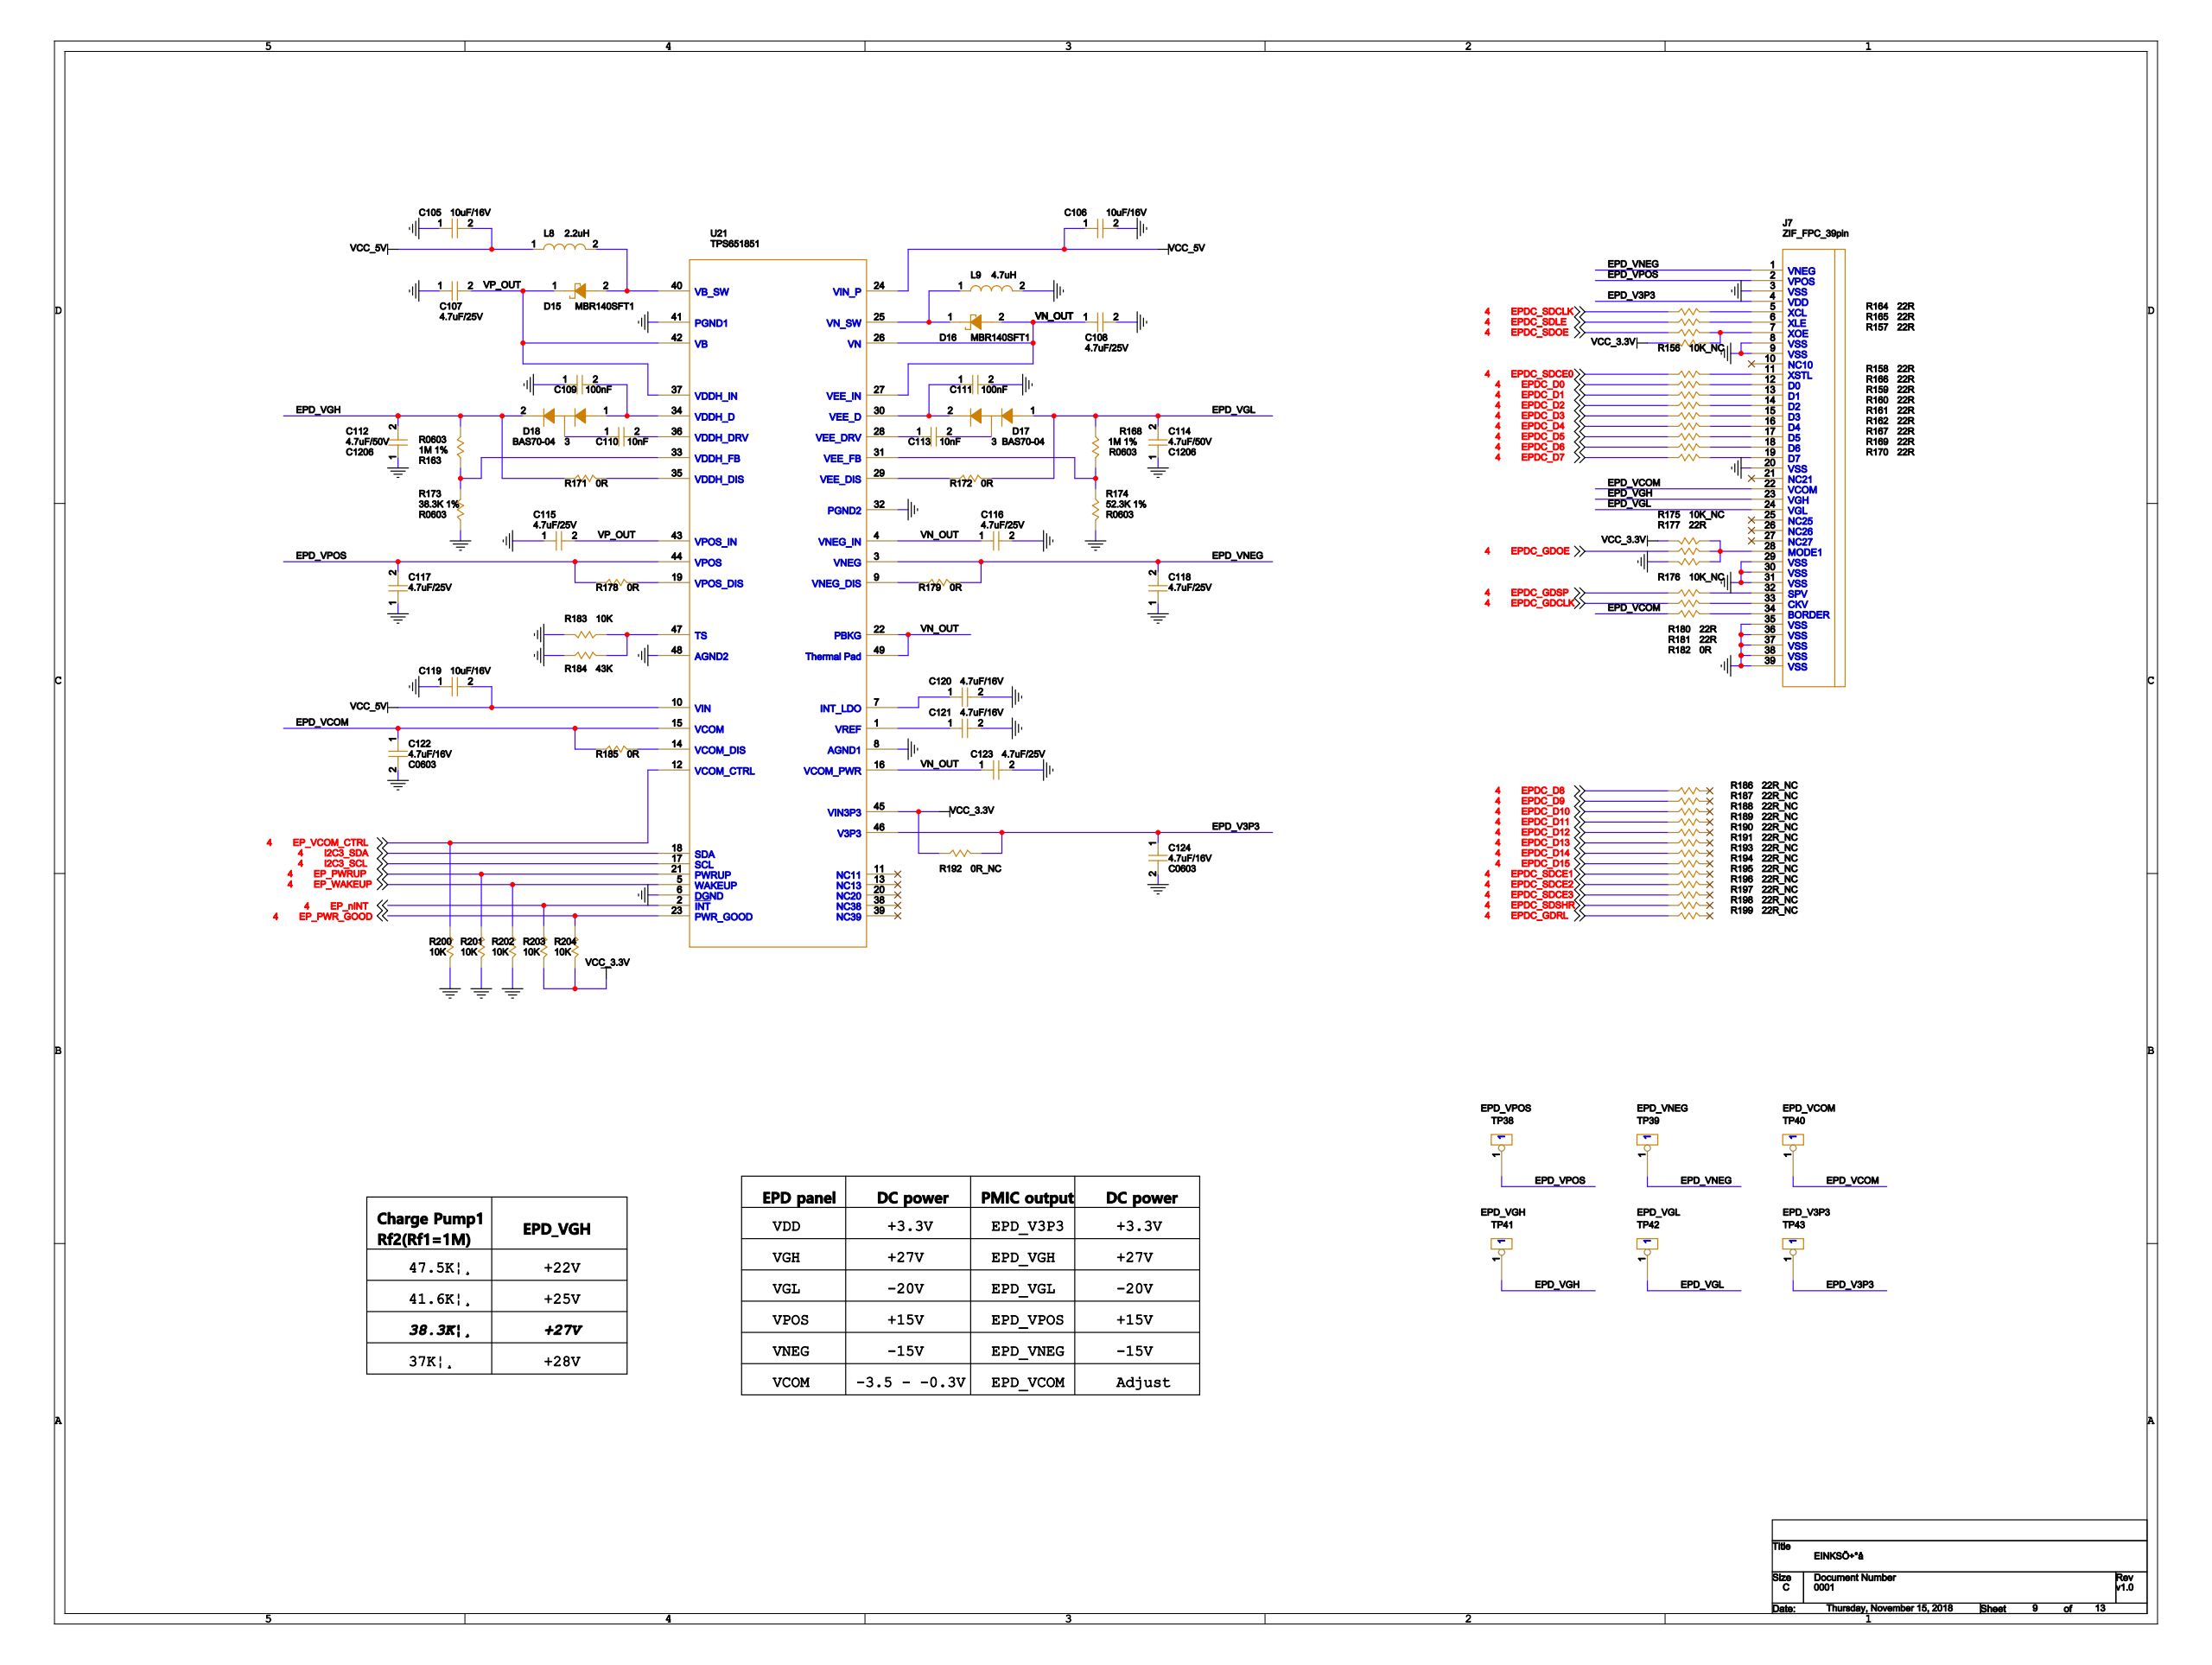Circuit board | Cadence Allegro | 609 parts | 409 nets | one sheet of the schematic
Parts on this sheet (reference | value | footprint):
C105 | 10uF/16V | C1206
C106 | 10uF/16V | C1206
C107 | 4.7uF/25V | C0805
C108 | 4.7uF/25V | C0805
C109 | 100nF | C0603
C110 | 10nF | C0603
C111 | 100nF | C0603
C112 | 4.7uF/50V | C1206
C113 | 10nF | C0603
C114 | 4.7uF/50V | C1206
C115 | 4.7uF/25V | C0805
C116 | 4.7uF/25V | C0805
C117 | 4.7uF/25V | C0805
C118 | 4.7uF/25V | C0805
C119 | 10uF/16V | C1206
C120 | 4.7uF/16V | C0603
C121 | 4.7uF/16V | C0603
C122 | 4.7uF/16V | C0603
C123 | 4.7uF/25V | C0805
C124 | 4.7uF/16V | C0603
D15 | MBR140SFT1 | SOD-123FL
D16 | MBR140SFT1 | SOD-123FL
D17 | BAS70-04 | SOT23
D18 | BAS70-04 | SOT23
J7 | ZIF_FPC_39pin | 39FXL
L8 | 2.2uH | IND_VLS3012_SM
L9 | 4.7uH | IND_VLS3012_SM
R156 | 10K_NC | R0603
R157 | 22R | R0603
R158 | 22R | R0603
R159 | 22R | R0603
R160 | 22R | R0603
R161 | 22R | R0603
R162 | 22R | R0603
R163 | 1M 1% | R0603
R164 | 22R | R0603
R165 | 22R | R0603
R166 | 22R | R0603
R167 | 22R | R0603
R168 | 1M 1% | R0603
R169 | 22R | R0603
R170 | 22R | R0603
R171 | 0R | R0603
R172 | 0R | R0603
R173 | 38.3K 1% | R0603
R174 | 52.3K 1% | R0603
R175 | 10K_NC | R0603
R176 | 10K_NC | R0603
R177 | 22R | R0603
R178 | 0R | R0603
R179 | 0R | R0603
R180 | 22R | R0603
R181 | 22R | R0603
R182 | 0R | R0603
R183 | 10K | R0603
R184 | 43K | R0603
R185 | 0R | R0603
R186 | 22R_NC | R0603
R187 | 22R_NC | R0603
R188 | 22R_NC | R0603
R189 | 22R_NC | R0603
R190 | 22R_NC | R0603
R191 | 22R_NC | R0603
R192 | 0R_NC | R0603
R193 | 22R_NC | R0603
R194 | 22R_NC | R0603
R195 | 22R_NC | R0603
R196 | 22R_NC | R0603
R197 | 22R_NC | R0603
R198 | 22R_NC | R0603
R199 | 22R_NC | R0603
R200 | 10K | R0603
R201 | 10K | R0603
R202 | 10K | R0603
R203 | 10K | R0603
R204 | 10K | R0603
TP38 | EPD_VPOS | TP_50
TP39 | EPD_VNEG | TP_50
TP40 | EPD_VCOM | TP_50
TP41 | EPD_VGH | TP_50
TP42 | EPD_VGL | TP_50
TP43 | EPD_V3P3 | TP_50
U21 | TPS651851 | VQFN48P
Nets of these parts (net: part-pin ...):
GND: C105-1 C106-2 C107-1 C108-2 C109-1 C111-2 C112-1 C114-1 C115-1 C116-2 C117-1 C118-1 C119-1 C120-2 C121-2 C122-2 C123-2 C124-2 L9-2 R173-1 R174-1 R176-2 R183-2 R184-2 R200-2 R201-2 R202-2 J7-3 J7-8 J7-9 J7-20 J7-29 J7-30 J7-31 J7-35 J7-36 J7-37 J7-38 J7-39 U21-6 U21-8 U21-32 U21-41 U21-48
VP_OUT: C107-2 C115-2 D15-1 U21-37 U21-42 U21-43
VN_OUT: C108-1 C116-1 C123-1 D16-2 U21-4 U21-16 U21-22 U21-26 U21-27 U21-49
EPD_VPOS: C117-2 R178-2 TP38-1 J7-2 U21-44
EPD_VNEG: C118-2 R179-1 TP39-1 J7-1 U21-3
EPD_VGH: C112-2 D18-2 R163-1 R171-2 TP41-1 J7-23
EPD_VGL: C114-2 D17-1 R168-2 R172-1 TP42-1 J7-24
VCC_3.3V: R156-2 R175-2 R192-2 R203-2 R204-2 U21-45
VCC_5V: C105-2 C106-1 C119-2 L8-1 U21-10 U21-24
N29044070: C111-1 D17-2 U21-30
N29044303: C113-2 D17-3
N29007672: C109-2 D18-1 U21-34
N29008367: C110-1 D18-3
EP_NINT: R203-1 U21-2
EPDC_D14: R193-2
EPDC_D5: R167-2
EPDC_D6: R169-2
EPDC_D7: R170-2
EP_PWR_GOOD: R204-1 U21-23
EP_VCOM_CTRL: R200-1 U21-12
EP_PWRUP: R201-1 U21-21
EP_WAKEUP: R202-1 U21-5
I2C3_SCL: U21-17
I2C3_SDA: U21-18
EPDC_D15: R194-2
EPDC_D0: R166-2
EPDC_D1: R159-2
EPDC_D10: R188-2
EPDC_D11: R189-2
EPDC_D12: R190-2
EPDC_D13: R191-2
EPDC_D2: R160-2
EPDC_D3: R161-2
EPDC_D4: R162-2
EPDC_D8: R186-2
EPDC_D9: R187-2
EPDC_SDCE1: R195-2
EPDC_SDCLK: R164-2
EPDC_SDLE: R165-2
EPDC_SDOE: R157-2
EPDC_SDSHR: R198-2
EPDC_SDCE0: R158-2
EPDC_GDSP: R180-2
EPDC_SDCE2: R196-2
EPDC_SDCE3: R197-2
EPDC_GDCLK: R181-2
EPDC_GDOE: R177-2
EPDC_GDRL: R199-2
N29063044: R182-1 J7-34
N29063023: R181-1 J7-33
N29061294: R166-1 J7-12
N29061297: R159-1 J7-13
N29061300: R160-1 J7-14
N29061303: R161-1 J7-15
N29061306: R162-1 J7-16
N29061309: R167-1 J7-17
N29061312: R169-1 J7-18
N29061315: R170-1 J7-19
N29061903: R175-1 R176-1 R177-1 J7-28
N29063002: R180-1 J7-32
EPD_VCOM: C122-1 R182-2 R185-2 TP40-1 J7-22 U21-15
EPD_V3P3: C124-1 R192-1 TP43-1 J7-4 U21-46
N29061262: R164-1 J7-5
N29061259: R165-1 J7-6
N29061256: R156-1 R157-1 J7-7
N29061291: R158-1 J7-11
N29042539: D16-1 L9-1 U21-25
N29000257: D15-2 L8-2 U21-40
N29008706: R163-2 R173-2 U21-33
N29044390: R168-1 R174-2 U21-31
N29014637: R183-1 R184-1 U21-47
N29056424: C120-1 U21-7
N29012998: R185-1 U21-14
N29009774: R171-1 U21-35
N29008364: C110-2 U21-36
N29044369: R172-2 U21-29
N29044300: C113-1 U21-28
N29056038: R179-2 U21-9
N29010120: R178-1 U21-19
N29056417: C121-1 U21-1